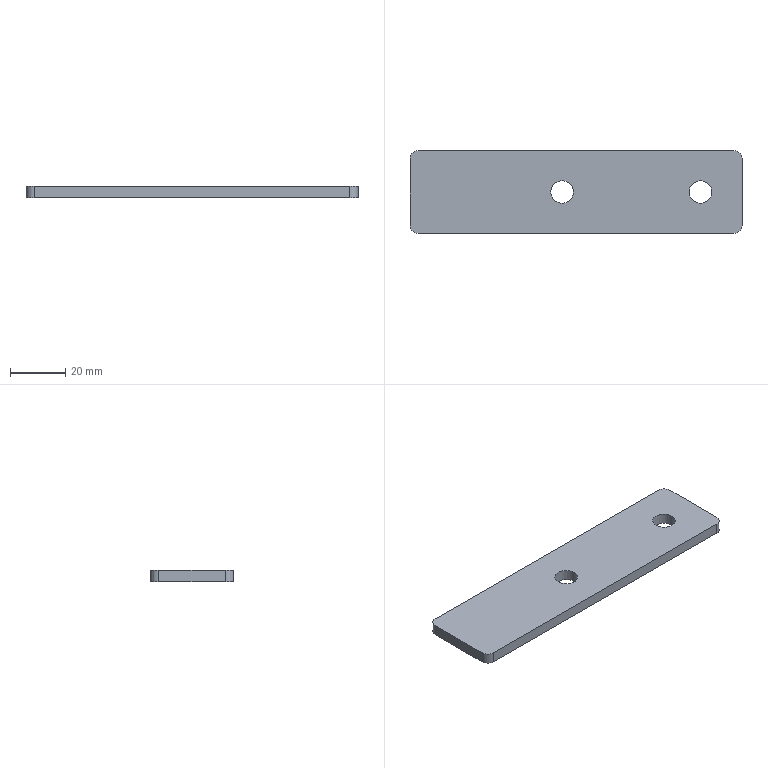Part | STEP file | Mounting bumper | 1 solid | 12 faces | box 120 x 30 x 4 mm | volume 13947 mm3 | cylinder 6 | plane 6 | commonest cylinder face diameters 6 x4 8.2 x2
STEP:
#1=CARTESIAN_POINT('',(0.,0.,0.));
#2=DIRECTION('',(0.,0.,1.));
#3=DIRECTION('',(1.,0.,0.));
#4=AXIS2_PLACEMENT_3D('',#1,#2,#3);
#5=CARTESIAN_POINT('',(109.1,15.,0.));
#6=VERTEX_POINT('',#5);
#7=CARTESIAN_POINT('',(105.,15.,0.));
#8=DIRECTION('',(0.,0.,1.));
#9=DIRECTION('',(-1.,0.,0.));
#10=AXIS2_PLACEMENT_3D('',#7,#8,#9);
#11=CIRCLE('',#10,4.1);
#12=CARTESIAN_POINT('',(105.,15.,4.));
#13=DIRECTION('',(0.,0.,-1.));
#14=DIRECTION('',(-1.,0.,0.));
#15=AXIS2_PLACEMENT_3D('',#12,#13,#14);
#16=CYLINDRICAL_SURFACE('',#15,4.1);
#17=CARTESIAN_POINT('',(12.566,4.));
#18=DIRECTION('',(-1.,0.));
#19=VECTOR('',#18,1.);
#20=LINE('',#17,#19);
#21=(GEOMETRIC_REPRESENTATION_CONTEXT(2)PARAMETRIC_REPRESENTATION_CONTEXT()REPRESENTATION_CONTEXT('',''));
#22=DEFINITIONAL_REPRESENTATION('',(#20),#21);
#23=PCURVE('',#16,#22);
#24=CARTESIAN_POINT('',(60.,15.,0.));
#25=DIRECTION('',(0.,0.,1.));
#26=DIRECTION('',(1.,0.,0.));
#27=AXIS2_PLACEMENT_3D('',#24,#25,#26);
#28=PLANE('',#27);
#29=CARTESIAN_POINT('',(45.,0.));
#30=DIRECTION('',(-1.,0.));
#31=AXIS2_PLACEMENT_2D('',#29,#30);
#32=CIRCLE('',#31,4.1);
#33=(GEOMETRIC_REPRESENTATION_CONTEXT(2)PARAMETRIC_REPRESENTATION_CONTEXT()REPRESENTATION_CONTEXT('',''));
#34=DEFINITIONAL_REPRESENTATION('',(#32),#33);
#35=PCURVE('',#28,#34);
#36=SURFACE_CURVE('',#11,(#23,#35),.PCURVE_S1.);
#37=EDGE_CURVE('',#6,#6,#36,.T.);
#38=ORIENTED_EDGE('',*,*,#37,.T.);
#39=CARTESIAN_POINT('',(109.1,15.,4.));
#40=VERTEX_POINT('',#39);
#41=CARTESIAN_POINT('',(109.1,15.,4.));
#42=CARTESIAN_POINT('',(109.1,15.,0.));
#43=B_SPLINE_CURVE_WITH_KNOTS('',1,(#41,#42),.UNSPECIFIED.,.F.,.F.,(2,2),(0.,4.),.PIECEWISE_BEZIER_KNOTS.);
#44=CARTESIAN_POINT('',(3.142,0.));
#45=DIRECTION('',(0.,1.));
#46=VECTOR('',#45,1.);
#47=LINE('',#44,#46);
#48=(GEOMETRIC_REPRESENTATION_CONTEXT(2)PARAMETRIC_REPRESENTATION_CONTEXT()REPRESENTATION_CONTEXT('',''));
#49=DEFINITIONAL_REPRESENTATION('',(#47),#48);
#50=PCURVE('',#16,#49);
#51=CARTESIAN_POINT('',(9.425,0.));
#52=DIRECTION('',(0.,1.));
#53=VECTOR('',#52,1.);
#54=LINE('',#51,#53);
#55=(GEOMETRIC_REPRESENTATION_CONTEXT(2)PARAMETRIC_REPRESENTATION_CONTEXT()REPRESENTATION_CONTEXT('',''));
#56=DEFINITIONAL_REPRESENTATION('',(#54),#55);
#57=PCURVE('',#16,#56);
#58=SEAM_CURVE('',#43,(#50,#57),.PCURVE_S1.);
#59=EDGE_CURVE('',#40,#6,#58,.T.);
#60=ORIENTED_EDGE('',*,*,#59,.F.);
#61=CARTESIAN_POINT('',(105.,15.,4.));
#62=DIRECTION('',(0.,0.,-1.));
#63=DIRECTION('',(-1.,0.,0.));
#64=AXIS2_PLACEMENT_3D('',#61,#62,#63);
#65=CIRCLE('',#64,4.1);
#66=CARTESIAN_POINT('',(0.,0.));
#67=DIRECTION('',(1.,0.));
#68=VECTOR('',#67,1.);
#69=LINE('',#66,#68);
#70=(GEOMETRIC_REPRESENTATION_CONTEXT(2)PARAMETRIC_REPRESENTATION_CONTEXT()REPRESENTATION_CONTEXT('',''));
#71=DEFINITIONAL_REPRESENTATION('',(#69),#70);
#72=PCURVE('',#16,#71);
#73=CARTESIAN_POINT('',(60.,15.,4.));
#74=DIRECTION('',(0.,0.,1.));
#75=DIRECTION('',(1.,0.,0.));
#76=AXIS2_PLACEMENT_3D('',#73,#74,#75);
#77=PLANE('',#76);
#78=CARTESIAN_POINT('',(40.9,0.));
#79=CARTESIAN_POINT('',(40.9,7.101));
#80=CARTESIAN_POINT('',(47.05,3.551));
#81=CARTESIAN_POINT('',(53.2,0.));
#82=CARTESIAN_POINT('',(47.05,-3.551));
#83=CARTESIAN_POINT('',(40.9,-7.101));
#84=CARTESIAN_POINT('',(40.9,0.));
#85=(BOUNDED_CURVE()B_SPLINE_CURVE(2,(#78,#79,#80,#81,#82,#83,#84),.UNSPECIFIED.,.T.,.F.)B_SPLINE_CURVE_WITH_KNOTS((1,2,2,2,2,1),(-2.094,0.,2.094,4.189,6.283,8.378),.UNSPECIFIED.)CURVE()GEOMETRIC_REPRESENTATION_ITEM()RATIONAL_B_SPLINE_CURVE((1.,0.5,1.,0.5,1.,0.5,1.))REPRESENTATION_ITEM(''));
#86=(GEOMETRIC_REPRESENTATION_CONTEXT(2)PARAMETRIC_REPRESENTATION_CONTEXT()REPRESENTATION_CONTEXT('',''));
#87=DEFINITIONAL_REPRESENTATION('',(#85),#86);
#88=PCURVE('',#77,#87);
#89=SURFACE_CURVE('',#65,(#72,#88),.PCURVE_S1.);
#90=EDGE_CURVE('',#40,#40,#89,.T.);
#91=ORIENTED_EDGE('',*,*,#90,.T.);
#92=ORIENTED_EDGE('',*,*,#59,.T.);
#93=EDGE_LOOP('',(#38,#60,#91,#92));
#94=FACE_BOUND('',#93,.F.);
#95=ADVANCED_FACE('',(#94),#16,.F.);
#96=CARTESIAN_POINT('',(59.1,15.,0.));
#97=VERTEX_POINT('',#96);
#98=CARTESIAN_POINT('',(55.,15.,0.));
#99=DIRECTION('',(0.,0.,1.));
#100=DIRECTION('',(-1.,0.,0.));
#101=AXIS2_PLACEMENT_3D('',#98,#99,#100);
#102=CIRCLE('',#101,4.1);
#103=CARTESIAN_POINT('',(55.,15.,4.));
#104=DIRECTION('',(0.,0.,-1.));
#105=DIRECTION('',(-1.,0.,0.));
#106=AXIS2_PLACEMENT_3D('',#103,#104,#105);
#107=CYLINDRICAL_SURFACE('',#106,4.1);
#108=CARTESIAN_POINT('',(12.566,4.));
#109=DIRECTION('',(-1.,0.));
#110=VECTOR('',#109,1.);
#111=LINE('',#108,#110);
#112=(GEOMETRIC_REPRESENTATION_CONTEXT(2)PARAMETRIC_REPRESENTATION_CONTEXT()REPRESENTATION_CONTEXT('',''));
#113=DEFINITIONAL_REPRESENTATION('',(#111),#112);
#114=PCURVE('',#107,#113);
#115=CARTESIAN_POINT('',(-5.,0.));
#116=DIRECTION('',(-1.,0.));
#117=AXIS2_PLACEMENT_2D('',#115,#116);
#118=CIRCLE('',#117,4.1);
#119=(GEOMETRIC_REPRESENTATION_CONTEXT(2)PARAMETRIC_REPRESENTATION_CONTEXT()REPRESENTATION_CONTEXT('',''));
#120=DEFINITIONAL_REPRESENTATION('',(#118),#119);
#121=PCURVE('',#28,#120);
#122=SURFACE_CURVE('',#102,(#114,#121),.PCURVE_S1.);
#123=EDGE_CURVE('',#97,#97,#122,.T.);
#124=ORIENTED_EDGE('',*,*,#123,.T.);
#125=CARTESIAN_POINT('',(59.1,15.,4.));
#126=VERTEX_POINT('',#125);
#127=CARTESIAN_POINT('',(59.1,15.,4.));
#128=CARTESIAN_POINT('',(59.1,15.,0.));
#129=B_SPLINE_CURVE_WITH_KNOTS('',1,(#127,#128),.UNSPECIFIED.,.F.,.F.,(2,2),(0.,4.),.PIECEWISE_BEZIER_KNOTS.);
#130=CARTESIAN_POINT('',(3.142,0.));
#131=DIRECTION('',(0.,1.));
#132=VECTOR('',#131,1.);
#133=LINE('',#130,#132);
#134=(GEOMETRIC_REPRESENTATION_CONTEXT(2)PARAMETRIC_REPRESENTATION_CONTEXT()REPRESENTATION_CONTEXT('',''));
#135=DEFINITIONAL_REPRESENTATION('',(#133),#134);
#136=PCURVE('',#107,#135);
#137=CARTESIAN_POINT('',(9.425,0.));
#138=DIRECTION('',(0.,1.));
#139=VECTOR('',#138,1.);
#140=LINE('',#137,#139);
#141=(GEOMETRIC_REPRESENTATION_CONTEXT(2)PARAMETRIC_REPRESENTATION_CONTEXT()REPRESENTATION_CONTEXT('',''));
#142=DEFINITIONAL_REPRESENTATION('',(#140),#141);
#143=PCURVE('',#107,#142);
#144=SEAM_CURVE('',#129,(#136,#143),.PCURVE_S1.);
#145=EDGE_CURVE('',#126,#97,#144,.T.);
#146=ORIENTED_EDGE('',*,*,#145,.F.);
#147=CARTESIAN_POINT('',(55.,15.,4.));
#148=DIRECTION('',(0.,0.,-1.));
#149=DIRECTION('',(-1.,0.,0.));
#150=AXIS2_PLACEMENT_3D('',#147,#148,#149);
#151=CIRCLE('',#150,4.1);
#152=CARTESIAN_POINT('',(0.,0.));
#153=DIRECTION('',(1.,0.));
#154=VECTOR('',#153,1.);
#155=LINE('',#152,#154);
#156=(GEOMETRIC_REPRESENTATION_CONTEXT(2)PARAMETRIC_REPRESENTATION_CONTEXT()REPRESENTATION_CONTEXT('',''));
#157=DEFINITIONAL_REPRESENTATION('',(#155),#156);
#158=PCURVE('',#107,#157);
#159=CARTESIAN_POINT('',(-9.1,0.));
#160=CARTESIAN_POINT('',(-9.1,7.101));
#161=CARTESIAN_POINT('',(-2.95,3.551));
#162=CARTESIAN_POINT('',(3.2,0.));
#163=CARTESIAN_POINT('',(-2.95,-3.551));
#164=CARTESIAN_POINT('',(-9.1,-7.101));
#165=CARTESIAN_POINT('',(-9.1,0.));
#166=(BOUNDED_CURVE()B_SPLINE_CURVE(2,(#159,#160,#161,#162,#163,#164,#165),.UNSPECIFIED.,.T.,.F.)B_SPLINE_CURVE_WITH_KNOTS((1,2,2,2,2,1),(-2.094,0.,2.094,4.189,6.283,8.378),.UNSPECIFIED.)CURVE()GEOMETRIC_REPRESENTATION_ITEM()RATIONAL_B_SPLINE_CURVE((1.,0.5,1.,0.5,1.,0.5,1.))REPRESENTATION_ITEM(''));
#167=(GEOMETRIC_REPRESENTATION_CONTEXT(2)PARAMETRIC_REPRESENTATION_CONTEXT()REPRESENTATION_CONTEXT('',''));
#168=DEFINITIONAL_REPRESENTATION('',(#166),#167);
#169=PCURVE('',#77,#168);
#170=SURFACE_CURVE('',#151,(#158,#169),.PCURVE_S1.);
#171=EDGE_CURVE('',#126,#126,#170,.T.);
#172=ORIENTED_EDGE('',*,*,#171,.T.);
#173=ORIENTED_EDGE('',*,*,#145,.T.);
#174=EDGE_LOOP('',(#124,#146,#172,#173));
#175=FACE_BOUND('',#174,.F.);
#176=ADVANCED_FACE('',(#175),#107,.F.);
#177=CARTESIAN_POINT('',(120.,3.,4.));
#178=VERTEX_POINT('',#177);
#179=CARTESIAN_POINT('',(117.,0.,4.));
#180=VERTEX_POINT('',#179);
#181=CARTESIAN_POINT('',(117.,3.,4.));
#182=DIRECTION('',(0.,0.,-1.));
#183=DIRECTION('',(0.7071,-0.7071,0.));
#184=AXIS2_PLACEMENT_3D('',#181,#182,#183);
#185=CIRCLE('',#184,3.);
#186=CARTESIAN_POINT('',(117.,3.,0.));
#187=DIRECTION('',(0.,0.,1.));
#188=DIRECTION('',(0.7071,-0.7071,0.));
#189=AXIS2_PLACEMENT_3D('',#186,#187,#188);
#190=CYLINDRICAL_SURFACE('',#189,3.);
#191=CARTESIAN_POINT('',(6.283,4.));
#192=DIRECTION('',(-1.,0.));
#193=VECTOR('',#192,1.);
#194=LINE('',#191,#193);
#195=(GEOMETRIC_REPRESENTATION_CONTEXT(2)PARAMETRIC_REPRESENTATION_CONTEXT()REPRESENTATION_CONTEXT('',''));
#196=DEFINITIONAL_REPRESENTATION('',(#194),#195);
#197=PCURVE('',#190,#196);
#198=CARTESIAN_POINT('',(59.121,-14.121));
#199=CARTESIAN_POINT('',(55.447,-17.796));
#200=CARTESIAN_POINT('',(54.102,-12.776));
#201=CARTESIAN_POINT('',(52.757,-7.757));
#202=CARTESIAN_POINT('',(57.776,-9.102));
#203=CARTESIAN_POINT('',(62.796,-10.447));
#204=CARTESIAN_POINT('',(59.121,-14.121));
#205=(BOUNDED_CURVE()B_SPLINE_CURVE(2,(#198,#199,#200,#201,#202,#203,#204),.UNSPECIFIED.,.T.,.F.)B_SPLINE_CURVE_WITH_KNOTS((1,2,2,2,2,1),(-2.094,0.,2.094,4.189,6.283,8.378),.UNSPECIFIED.)CURVE()GEOMETRIC_REPRESENTATION_ITEM()RATIONAL_B_SPLINE_CURVE((1.,0.5,1.,0.5,1.,0.5,1.))REPRESENTATION_ITEM(''));
#206=(GEOMETRIC_REPRESENTATION_CONTEXT(2)PARAMETRIC_REPRESENTATION_CONTEXT()REPRESENTATION_CONTEXT('',''));
#207=DEFINITIONAL_REPRESENTATION('',(#205),#206);
#208=PCURVE('',#77,#207);
#209=SURFACE_CURVE('',#185,(#197,#208),.PCURVE_S1.);
#210=EDGE_CURVE('',#178,#180,#209,.T.);
#211=ORIENTED_EDGE('',*,*,#210,.T.);
#212=CARTESIAN_POINT('',(117.,0.,0.));
#213=VERTEX_POINT('',#212);
#214=CARTESIAN_POINT('',(117.,0.,0.));
#215=DIRECTION('',(0.,0.,-1.));
#216=VECTOR('',#215,1.);
#217=LINE('',#214,#216);
#218=CARTESIAN_POINT('',(-0.7854,0.));
#219=DIRECTION('',(0.,-1.));
#220=VECTOR('',#219,1.);
#221=LINE('',#218,#220);
#222=(GEOMETRIC_REPRESENTATION_CONTEXT(2)PARAMETRIC_REPRESENTATION_CONTEXT()REPRESENTATION_CONTEXT('',''));
#223=DEFINITIONAL_REPRESENTATION('',(#221),#222);
#224=PCURVE('',#190,#223);
#225=CARTESIAN_POINT('',(120.,0.,0.));
#226=DIRECTION('',(0.,-1.,0.));
#227=DIRECTION('',(0.,0.,-1.));
#228=AXIS2_PLACEMENT_3D('',#225,#226,#227);
#229=PLANE('',#228);
#230=CARTESIAN_POINT('',(0.,-3.));
#231=DIRECTION('',(1.,0.));
#232=VECTOR('',#231,1.);
#233=LINE('',#230,#232);
#234=(GEOMETRIC_REPRESENTATION_CONTEXT(2)PARAMETRIC_REPRESENTATION_CONTEXT()REPRESENTATION_CONTEXT('',''));
#235=DEFINITIONAL_REPRESENTATION('',(#233),#234);
#236=PCURVE('',#229,#235);
#237=SURFACE_CURVE('',#217,(#224,#236),.PCURVE_S1.);
#238=EDGE_CURVE('',#180,#213,#237,.T.);
#239=ORIENTED_EDGE('',*,*,#238,.T.);
#240=CARTESIAN_POINT('',(120.,3.,0.));
#241=VERTEX_POINT('',#240);
#242=CARTESIAN_POINT('',(117.,3.,0.));
#243=DIRECTION('',(0.,0.,1.));
#244=DIRECTION('',(0.7071,-0.7071,0.));
#245=AXIS2_PLACEMENT_3D('',#242,#243,#244);
#246=CIRCLE('',#245,3.);
#247=CARTESIAN_POINT('',(-6.283,0.));
#248=DIRECTION('',(1.,0.));
#249=VECTOR('',#248,1.);
#250=LINE('',#247,#249);
#251=(GEOMETRIC_REPRESENTATION_CONTEXT(2)PARAMETRIC_REPRESENTATION_CONTEXT()REPRESENTATION_CONTEXT('',''));
#252=DEFINITIONAL_REPRESENTATION('',(#250),#251);
#253=PCURVE('',#190,#252);
#254=CARTESIAN_POINT('',(57.,-12.));
#255=DIRECTION('',(0.7071,-0.7071));
#256=AXIS2_PLACEMENT_2D('',#254,#255);
#257=CIRCLE('',#256,3.);
#258=(GEOMETRIC_REPRESENTATION_CONTEXT(2)PARAMETRIC_REPRESENTATION_CONTEXT()REPRESENTATION_CONTEXT('',''));
#259=DEFINITIONAL_REPRESENTATION('',(#257),#258);
#260=PCURVE('',#28,#259);
#261=SURFACE_CURVE('',#246,(#253,#260),.PCURVE_S1.);
#262=EDGE_CURVE('',#213,#241,#261,.T.);
#263=ORIENTED_EDGE('',*,*,#262,.T.);
#264=CARTESIAN_POINT('',(120.,3.,0.));
#265=DIRECTION('',(0.,0.,1.));
#266=VECTOR('',#265,1.);
#267=LINE('',#264,#266);
#268=CARTESIAN_POINT('',(0.7854,0.));
#269=DIRECTION('',(0.,1.));
#270=VECTOR('',#269,1.);
#271=LINE('',#268,#270);
#272=(GEOMETRIC_REPRESENTATION_CONTEXT(2)PARAMETRIC_REPRESENTATION_CONTEXT()REPRESENTATION_CONTEXT('',''));
#273=DEFINITIONAL_REPRESENTATION('',(#271),#272);
#274=PCURVE('',#190,#273);
#275=CARTESIAN_POINT('',(120.,30.,0.));
#276=DIRECTION('',(1.,0.,0.));
#277=DIRECTION('',(0.,0.,-1.));
#278=AXIS2_PLACEMENT_3D('',#275,#276,#277);
#279=PLANE('',#278);
#280=CARTESIAN_POINT('',(0.,-27.));
#281=DIRECTION('',(-1.,0.));
#282=VECTOR('',#281,1.);
#283=LINE('',#280,#282);
#284=(GEOMETRIC_REPRESENTATION_CONTEXT(2)PARAMETRIC_REPRESENTATION_CONTEXT()REPRESENTATION_CONTEXT('',''));
#285=DEFINITIONAL_REPRESENTATION('',(#283),#284);
#286=PCURVE('',#279,#285);
#287=SURFACE_CURVE('',#267,(#274,#286),.PCURVE_S1.);
#288=EDGE_CURVE('',#241,#178,#287,.T.);
#289=ORIENTED_EDGE('',*,*,#288,.T.);
#290=EDGE_LOOP('',(#211,#239,#263,#289));
#291=FACE_BOUND('',#290,.T.);
#292=ADVANCED_FACE('',(#291),#190,.T.);
#293=ORIENTED_EDGE('',*,*,#288,.F.);
#294=CARTESIAN_POINT('',(120.,27.,0.));
#295=VERTEX_POINT('',#294);
#296=CARTESIAN_POINT('',(120.,30.,0.));
#297=DIRECTION('',(0.,-1.,0.));
#298=VECTOR('',#297,1.);
#299=LINE('',#296,#298);
#300=CARTESIAN_POINT('',(0.,0.));
#301=DIRECTION('',(0.,-1.));
#302=VECTOR('',#301,1.);
#303=LINE('',#300,#302);
#304=(GEOMETRIC_REPRESENTATION_CONTEXT(2)PARAMETRIC_REPRESENTATION_CONTEXT()REPRESENTATION_CONTEXT('',''));
#305=DEFINITIONAL_REPRESENTATION('',(#303),#304);
#306=PCURVE('',#279,#305);
#307=CARTESIAN_POINT('',(60.,15.));
#308=DIRECTION('',(0.,-1.));
#309=VECTOR('',#308,1.);
#310=LINE('',#307,#309);
#311=(GEOMETRIC_REPRESENTATION_CONTEXT(2)PARAMETRIC_REPRESENTATION_CONTEXT()REPRESENTATION_CONTEXT('',''));
#312=DEFINITIONAL_REPRESENTATION('',(#310),#311);
#313=PCURVE('',#28,#312);
#314=SURFACE_CURVE('',#299,(#306,#313),.PCURVE_S1.);
#315=EDGE_CURVE('',#295,#241,#314,.T.);
#316=ORIENTED_EDGE('',*,*,#315,.F.);
#317=CARTESIAN_POINT('',(120.,27.,4.));
#318=VERTEX_POINT('',#317);
#319=CARTESIAN_POINT('',(120.,27.,0.));
#320=DIRECTION('',(0.,0.,-1.));
#321=VECTOR('',#320,1.);
#322=LINE('',#319,#321);
#323=CARTESIAN_POINT('',(0.,-3.));
#324=DIRECTION('',(1.,0.));
#325=VECTOR('',#324,1.);
#326=LINE('',#323,#325);
#327=(GEOMETRIC_REPRESENTATION_CONTEXT(2)PARAMETRIC_REPRESENTATION_CONTEXT()REPRESENTATION_CONTEXT('',''));
#328=DEFINITIONAL_REPRESENTATION('',(#326),#327);
#329=PCURVE('',#279,#328);
#330=CARTESIAN_POINT('',(117.,27.,0.));
#331=DIRECTION('',(0.,0.,1.));
#332=DIRECTION('',(0.7071,0.7071,0.));
#333=AXIS2_PLACEMENT_3D('',#330,#331,#332);
#334=CYLINDRICAL_SURFACE('',#333,3.);
#335=CARTESIAN_POINT('',(-0.7854,0.));
#336=DIRECTION('',(0.,-1.));
#337=VECTOR('',#336,1.);
#338=LINE('',#335,#337);
#339=(GEOMETRIC_REPRESENTATION_CONTEXT(2)PARAMETRIC_REPRESENTATION_CONTEXT()REPRESENTATION_CONTEXT('',''));
#340=DEFINITIONAL_REPRESENTATION('',(#338),#339);
#341=PCURVE('',#334,#340);
#342=SURFACE_CURVE('',#322,(#329,#341),.PCURVE_S1.);
#343=EDGE_CURVE('',#318,#295,#342,.T.);
#344=ORIENTED_EDGE('',*,*,#343,.F.);
#345=CARTESIAN_POINT('',(120.,30.,4.));
#346=DIRECTION('',(0.,-1.,0.));
#347=VECTOR('',#346,1.);
#348=LINE('',#345,#347);
#349=CARTESIAN_POINT('',(-4.,0.));
#350=DIRECTION('',(0.,-1.));
#351=VECTOR('',#350,1.);
#352=LINE('',#349,#351);
#353=(GEOMETRIC_REPRESENTATION_CONTEXT(2)PARAMETRIC_REPRESENTATION_CONTEXT()REPRESENTATION_CONTEXT('',''));
#354=DEFINITIONAL_REPRESENTATION('',(#352),#353);
#355=PCURVE('',#279,#354);
#356=CARTESIAN_POINT('',(60.,15.));
#357=DIRECTION('',(0.,-1.));
#358=VECTOR('',#357,1.);
#359=LINE('',#356,#358);
#360=(GEOMETRIC_REPRESENTATION_CONTEXT(2)PARAMETRIC_REPRESENTATION_CONTEXT()REPRESENTATION_CONTEXT('',''));
#361=DEFINITIONAL_REPRESENTATION('',(#359),#360);
#362=PCURVE('',#77,#361);
#363=SURFACE_CURVE('',#348,(#355,#362),.PCURVE_S1.);
#364=EDGE_CURVE('',#318,#178,#363,.T.);
#365=ORIENTED_EDGE('',*,*,#364,.T.);
#366=EDGE_LOOP('',(#293,#316,#344,#365));
#367=FACE_BOUND('',#366,.T.);
#368=ADVANCED_FACE('',(#367),#279,.T.);
#369=ORIENTED_EDGE('',*,*,#262,.F.);
#370=CARTESIAN_POINT('',(3.,0.,0.));
#371=VERTEX_POINT('',#370);
#372=CARTESIAN_POINT('',(120.,0.,0.));
#373=DIRECTION('',(-1.,0.,0.));
#374=VECTOR('',#373,1.);
#375=LINE('',#372,#374);
#376=CARTESIAN_POINT('',(60.,-15.));
#377=DIRECTION('',(-1.,0.));
#378=VECTOR('',#377,1.);
#379=LINE('',#376,#378);
#380=(GEOMETRIC_REPRESENTATION_CONTEXT(2)PARAMETRIC_REPRESENTATION_CONTEXT()REPRESENTATION_CONTEXT('',''));
#381=DEFINITIONAL_REPRESENTATION('',(#379),#380);
#382=PCURVE('',#28,#381);
#383=CARTESIAN_POINT('',(0.,0.));
#384=DIRECTION('',(0.,-1.));
#385=VECTOR('',#384,1.);
#386=LINE('',#383,#385);
#387=(GEOMETRIC_REPRESENTATION_CONTEXT(2)PARAMETRIC_REPRESENTATION_CONTEXT()REPRESENTATION_CONTEXT('',''));
#388=DEFINITIONAL_REPRESENTATION('',(#386),#387);
#389=PCURVE('',#229,#388);
#390=SURFACE_CURVE('',#375,(#382,#389),.PCURVE_S1.);
#391=EDGE_CURVE('',#213,#371,#390,.T.);
#392=ORIENTED_EDGE('',*,*,#391,.T.);
#393=CARTESIAN_POINT('',(0.,3.,0.));
#394=VERTEX_POINT('',#393);
#395=CARTESIAN_POINT('',(3.,3.,0.));
#396=DIRECTION('',(0.,0.,1.));
#397=DIRECTION('',(-0.7071,-0.7071,0.));
#398=AXIS2_PLACEMENT_3D('',#395,#396,#397);
#399=CIRCLE('',#398,3.);
#400=CARTESIAN_POINT('',(-57.,-12.));
#401=DIRECTION('',(-0.7071,-0.7071));
#402=AXIS2_PLACEMENT_2D('',#400,#401);
#403=CIRCLE('',#402,3.);
#404=(GEOMETRIC_REPRESENTATION_CONTEXT(2)PARAMETRIC_REPRESENTATION_CONTEXT()REPRESENTATION_CONTEXT('',''));
#405=DEFINITIONAL_REPRESENTATION('',(#403),#404);
#406=PCURVE('',#28,#405);
#407=CARTESIAN_POINT('',(3.,3.,0.));
#408=DIRECTION('',(0.,0.,1.));
#409=DIRECTION('',(-0.7071,-0.7071,0.));
#410=AXIS2_PLACEMENT_3D('',#407,#408,#409);
#411=CYLINDRICAL_SURFACE('',#410,3.);
#412=CARTESIAN_POINT('',(-6.283,0.));
#413=DIRECTION('',(1.,0.));
#414=VECTOR('',#413,1.);
#415=LINE('',#412,#414);
#416=(GEOMETRIC_REPRESENTATION_CONTEXT(2)PARAMETRIC_REPRESENTATION_CONTEXT()REPRESENTATION_CONTEXT('',''));
#417=DEFINITIONAL_REPRESENTATION('',(#415),#416);
#418=PCURVE('',#411,#417);
#419=SURFACE_CURVE('',#399,(#406,#418),.PCURVE_S1.);
#420=EDGE_CURVE('',#394,#371,#419,.T.);
#421=ORIENTED_EDGE('',*,*,#420,.F.);
#422=CARTESIAN_POINT('',(0.,27.,0.));
#423=VERTEX_POINT('',#422);
#424=CARTESIAN_POINT('',(0.,0.,0.));
#425=DIRECTION('',(0.,1.,0.));
#426=VECTOR('',#425,1.);
#427=LINE('',#424,#426);
#428=CARTESIAN_POINT('',(-60.,-15.));
#429=DIRECTION('',(0.,1.));
#430=VECTOR('',#429,1.);
#431=LINE('',#428,#430);
#432=(GEOMETRIC_REPRESENTATION_CONTEXT(2)PARAMETRIC_REPRESENTATION_CONTEXT()REPRESENTATION_CONTEXT('',''));
#433=DEFINITIONAL_REPRESENTATION('',(#431),#432);
#434=PCURVE('',#28,#433);
#435=CARTESIAN_POINT('',(0.,0.,0.));
#436=DIRECTION('',(-1.,0.,0.));
#437=DIRECTION('',(0.,0.,1.));
#438=AXIS2_PLACEMENT_3D('',#435,#436,#437);
#439=PLANE('',#438);
#440=CARTESIAN_POINT('',(0.,0.));
#441=DIRECTION('',(0.,1.));
#442=VECTOR('',#441,1.);
#443=LINE('',#440,#442);
#444=(GEOMETRIC_REPRESENTATION_CONTEXT(2)PARAMETRIC_REPRESENTATION_CONTEXT()REPRESENTATION_CONTEXT('',''));
#445=DEFINITIONAL_REPRESENTATION('',(#443),#444);
#446=PCURVE('',#439,#445);
#447=SURFACE_CURVE('',#427,(#434,#446),.PCURVE_S1.);
#448=EDGE_CURVE('',#394,#423,#447,.T.);
#449=ORIENTED_EDGE('',*,*,#448,.T.);
#450=CARTESIAN_POINT('',(3.,30.,0.));
#451=VERTEX_POINT('',#450);
#452=CARTESIAN_POINT('',(3.,27.,0.));
#453=DIRECTION('',(0.,0.,1.));
#454=DIRECTION('',(-0.7071,0.7071,0.));
#455=AXIS2_PLACEMENT_3D('',#452,#453,#454);
#456=CIRCLE('',#455,3.);
#457=CARTESIAN_POINT('',(-57.,12.));
#458=DIRECTION('',(-0.7071,0.7071));
#459=AXIS2_PLACEMENT_2D('',#457,#458);
#460=CIRCLE('',#459,3.);
#461=(GEOMETRIC_REPRESENTATION_CONTEXT(2)PARAMETRIC_REPRESENTATION_CONTEXT()REPRESENTATION_CONTEXT('',''));
#462=DEFINITIONAL_REPRESENTATION('',(#460),#461);
#463=PCURVE('',#28,#462);
#464=CARTESIAN_POINT('',(3.,27.,0.));
#465=DIRECTION('',(0.,0.,1.));
#466=DIRECTION('',(-0.7071,0.7071,0.));
#467=AXIS2_PLACEMENT_3D('',#464,#465,#466);
#468=CYLINDRICAL_SURFACE('',#467,3.);
#469=CARTESIAN_POINT('',(0.,0.));
#470=DIRECTION('',(1.,0.));
#471=VECTOR('',#470,1.);
#472=LINE('',#469,#471);
#473=(GEOMETRIC_REPRESENTATION_CONTEXT(2)PARAMETRIC_REPRESENTATION_CONTEXT()REPRESENTATION_CONTEXT('',''));
#474=DEFINITIONAL_REPRESENTATION('',(#472),#473);
#475=PCURVE('',#468,#474);
#476=SURFACE_CURVE('',#456,(#463,#475),.PCURVE_S1.);
#477=EDGE_CURVE('',#451,#423,#476,.T.);
#478=ORIENTED_EDGE('',*,*,#477,.F.);
#479=CARTESIAN_POINT('',(117.,30.,0.));
#480=VERTEX_POINT('',#479);
#481=CARTESIAN_POINT('',(0.,30.,0.));
#482=DIRECTION('',(1.,0.,0.));
#483=VECTOR('',#482,1.);
#484=LINE('',#481,#483);
#485=CARTESIAN_POINT('',(-60.,15.));
#486=DIRECTION('',(1.,0.));
#487=VECTOR('',#486,1.);
#488=LINE('',#485,#487);
#489=(GEOMETRIC_REPRESENTATION_CONTEXT(2)PARAMETRIC_REPRESENTATION_CONTEXT()REPRESENTATION_CONTEXT('',''));
#490=DEFINITIONAL_REPRESENTATION('',(#488),#489);
#491=PCURVE('',#28,#490);
#492=CARTESIAN_POINT('',(30.,30.,0.));
#493=DIRECTION('',(0.,1.,0.));
#494=DIRECTION('',(0.,0.,1.));
#495=AXIS2_PLACEMENT_3D('',#492,#493,#494);
#496=PLANE('',#495);
#497=CARTESIAN_POINT('',(0.,-30.));
#498=DIRECTION('',(0.,1.));
#499=VECTOR('',#498,1.);
#500=LINE('',#497,#499);
#501=(GEOMETRIC_REPRESENTATION_CONTEXT(2)PARAMETRIC_REPRESENTATION_CONTEXT()REPRESENTATION_CONTEXT('',''));
#502=DEFINITIONAL_REPRESENTATION('',(#500),#501);
#503=PCURVE('',#496,#502);
#504=SURFACE_CURVE('',#484,(#491,#503),.PCURVE_S1.);
#505=EDGE_CURVE('',#451,#480,#504,.T.);
#506=ORIENTED_EDGE('',*,*,#505,.T.);
#507=CARTESIAN_POINT('',(117.,27.,0.));
#508=DIRECTION('',(0.,0.,1.));
#509=DIRECTION('',(0.7071,0.7071,0.));
#510=AXIS2_PLACEMENT_3D('',#507,#508,#509);
#511=CIRCLE('',#510,3.);
#512=CARTESIAN_POINT('',(57.,12.));
#513=DIRECTION('',(0.7071,0.7071));
#514=AXIS2_PLACEMENT_2D('',#512,#513);
#515=CIRCLE('',#514,3.);
#516=(GEOMETRIC_REPRESENTATION_CONTEXT(2)PARAMETRIC_REPRESENTATION_CONTEXT()REPRESENTATION_CONTEXT('',''));
#517=DEFINITIONAL_REPRESENTATION('',(#515),#516);
#518=PCURVE('',#28,#517);
#519=CARTESIAN_POINT('',(-6.283,0.));
#520=DIRECTION('',(1.,0.));
#521=VECTOR('',#520,1.);
#522=LINE('',#519,#521);
#523=(GEOMETRIC_REPRESENTATION_CONTEXT(2)PARAMETRIC_REPRESENTATION_CONTEXT()REPRESENTATION_CONTEXT('',''));
#524=DEFINITIONAL_REPRESENTATION('',(#522),#523);
#525=PCURVE('',#334,#524);
#526=SURFACE_CURVE('',#511,(#518,#525),.PCURVE_S1.);
#527=EDGE_CURVE('',#295,#480,#526,.T.);
#528=ORIENTED_EDGE('',*,*,#527,.F.);
#529=ORIENTED_EDGE('',*,*,#315,.T.);
#530=EDGE_LOOP('',(#369,#392,#421,#449,#478,#506,#528,#529));
#531=FACE_BOUND('',#530,.T.);
#532=ORIENTED_EDGE('',*,*,#37,.T.);
#533=EDGE_LOOP('',(#532));
#534=FACE_BOUND('',#533,.T.);
#535=ORIENTED_EDGE('',*,*,#123,.T.);
#536=EDGE_LOOP('',(#535));
#537=FACE_BOUND('',#536,.T.);
#538=ADVANCED_FACE('',(#531,#534,#537),#28,.F.);
#539=CARTESIAN_POINT('',(117.,30.,4.));
#540=VERTEX_POINT('',#539);
#541=CARTESIAN_POINT('',(117.,27.,4.));
#542=DIRECTION('',(0.,0.,-1.));
#543=DIRECTION('',(0.7071,0.7071,0.));
#544=AXIS2_PLACEMENT_3D('',#541,#542,#543);
#545=CIRCLE('',#544,3.);
#546=CARTESIAN_POINT('',(6.283,4.));
#547=DIRECTION('',(-1.,0.));
#548=VECTOR('',#547,1.);
#549=LINE('',#546,#548);
#550=(GEOMETRIC_REPRESENTATION_CONTEXT(2)PARAMETRIC_REPRESENTATION_CONTEXT()REPRESENTATION_CONTEXT('',''));
#551=DEFINITIONAL_REPRESENTATION('',(#549),#550);
#552=PCURVE('',#334,#551);
#553=CARTESIAN_POINT('',(59.121,14.121));
#554=CARTESIAN_POINT('',(62.796,10.447));
#555=CARTESIAN_POINT('',(57.776,9.102));
#556=CARTESIAN_POINT('',(52.757,7.757));
#557=CARTESIAN_POINT('',(54.102,12.776));
#558=CARTESIAN_POINT('',(55.447,17.796));
#559=CARTESIAN_POINT('',(59.121,14.121));
#560=(BOUNDED_CURVE()B_SPLINE_CURVE(2,(#553,#554,#555,#556,#557,#558,#559),.UNSPECIFIED.,.T.,.F.)B_SPLINE_CURVE_WITH_KNOTS((1,2,2,2,2,1),(-2.094,0.,2.094,4.189,6.283,8.378),.UNSPECIFIED.)CURVE()GEOMETRIC_REPRESENTATION_ITEM()RATIONAL_B_SPLINE_CURVE((1.,0.5,1.,0.5,1.,0.5,1.))REPRESENTATION_ITEM(''));
#561=(GEOMETRIC_REPRESENTATION_CONTEXT(2)PARAMETRIC_REPRESENTATION_CONTEXT()REPRESENTATION_CONTEXT('',''));
#562=DEFINITIONAL_REPRESENTATION('',(#560),#561);
#563=PCURVE('',#77,#562);
#564=SURFACE_CURVE('',#545,(#552,#563),.PCURVE_S1.);
#565=EDGE_CURVE('',#540,#318,#564,.T.);
#566=ORIENTED_EDGE('',*,*,#565,.T.);
#567=ORIENTED_EDGE('',*,*,#343,.T.);
#568=ORIENTED_EDGE('',*,*,#527,.T.);
#569=CARTESIAN_POINT('',(117.,30.,0.));
#570=DIRECTION('',(0.,0.,1.));
#571=VECTOR('',#570,1.);
#572=LINE('',#569,#571);
#573=CARTESIAN_POINT('',(0.7854,0.));
#574=DIRECTION('',(0.,1.));
#575=VECTOR('',#574,1.);
#576=LINE('',#573,#575);
#577=(GEOMETRIC_REPRESENTATION_CONTEXT(2)PARAMETRIC_REPRESENTATION_CONTEXT()REPRESENTATION_CONTEXT('',''));
#578=DEFINITIONAL_REPRESENTATION('',(#576),#577);
#579=PCURVE('',#334,#578);
#580=CARTESIAN_POINT('',(0.,87.));
#581=DIRECTION('',(1.,0.));
#582=VECTOR('',#581,1.);
#583=LINE('',#580,#582);
#584=(GEOMETRIC_REPRESENTATION_CONTEXT(2)PARAMETRIC_REPRESENTATION_CONTEXT()REPRESENTATION_CONTEXT('',''));
#585=DEFINITIONAL_REPRESENTATION('',(#583),#584);
#586=PCURVE('',#496,#585);
#587=SURFACE_CURVE('',#572,(#579,#586),.PCURVE_S1.);
#588=EDGE_CURVE('',#480,#540,#587,.T.);
#589=ORIENTED_EDGE('',*,*,#588,.T.);
#590=EDGE_LOOP('',(#566,#567,#568,#589));
#591=FACE_BOUND('',#590,.T.);
#592=ADVANCED_FACE('',(#591),#334,.T.);
#593=ORIENTED_EDGE('',*,*,#588,.F.);
#594=ORIENTED_EDGE('',*,*,#505,.F.);
#595=CARTESIAN_POINT('',(3.,30.,4.));
#596=VERTEX_POINT('',#595);
#597=CARTESIAN_POINT('',(3.,30.,0.));
#598=DIRECTION('',(0.,0.,-1.));
#599=VECTOR('',#598,1.);
#600=LINE('',#597,#599);
#601=CARTESIAN_POINT('',(0.,-27.));
#602=DIRECTION('',(-1.,0.));
#603=VECTOR('',#602,1.);
#604=LINE('',#601,#603);
#605=(GEOMETRIC_REPRESENTATION_CONTEXT(2)PARAMETRIC_REPRESENTATION_CONTEXT()REPRESENTATION_CONTEXT('',''));
#606=DEFINITIONAL_REPRESENTATION('',(#604),#605);
#607=PCURVE('',#496,#606);
#608=CARTESIAN_POINT('',(5.498,0.));
#609=DIRECTION('',(0.,-1.));
#610=VECTOR('',#609,1.);
#611=LINE('',#608,#610);
#612=(GEOMETRIC_REPRESENTATION_CONTEXT(2)PARAMETRIC_REPRESENTATION_CONTEXT()REPRESENTATION_CONTEXT('',''));
#613=DEFINITIONAL_REPRESENTATION('',(#611),#612);
#614=PCURVE('',#468,#613);
#615=SURFACE_CURVE('',#600,(#607,#614),.PCURVE_S1.);
#616=EDGE_CURVE('',#596,#451,#615,.T.);
#617=ORIENTED_EDGE('',*,*,#616,.F.);
#618=CARTESIAN_POINT('',(30.,30.,4.));
#619=DIRECTION('',(1.,0.,0.));
#620=VECTOR('',#619,1.);
#621=LINE('',#618,#620);
#622=CARTESIAN_POINT('',(4.,0.));
#623=DIRECTION('',(0.,1.));
#624=VECTOR('',#623,1.);
#625=LINE('',#622,#624);
#626=(GEOMETRIC_REPRESENTATION_CONTEXT(2)PARAMETRIC_REPRESENTATION_CONTEXT()REPRESENTATION_CONTEXT('',''));
#627=DEFINITIONAL_REPRESENTATION('',(#625),#626);
#628=PCURVE('',#496,#627);
#629=CARTESIAN_POINT('',(-30.,15.));
#630=DIRECTION('',(1.,0.));
#631=VECTOR('',#630,1.);
#632=LINE('',#629,#631);
#633=(GEOMETRIC_REPRESENTATION_CONTEXT(2)PARAMETRIC_REPRESENTATION_CONTEXT()REPRESENTATION_CONTEXT('',''));
#634=DEFINITIONAL_REPRESENTATION('',(#632),#633);
#635=PCURVE('',#77,#634);
#636=SURFACE_CURVE('',#621,(#628,#635),.PCURVE_S1.);
#637=EDGE_CURVE('',#596,#540,#636,.T.);
#638=ORIENTED_EDGE('',*,*,#637,.T.);
#639=EDGE_LOOP('',(#593,#594,#617,#638));
#640=FACE_BOUND('',#639,.T.);
#641=ADVANCED_FACE('',(#640),#496,.T.);
#642=CARTESIAN_POINT('',(0.,27.,4.));
#643=VERTEX_POINT('',#642);
#644=CARTESIAN_POINT('',(3.,27.,4.));
#645=DIRECTION('',(0.,0.,-1.));
#646=DIRECTION('',(-0.7071,0.7071,0.));
#647=AXIS2_PLACEMENT_3D('',#644,#645,#646);
#648=CIRCLE('',#647,3.);
#649=CARTESIAN_POINT('',(12.566,4.));
#650=DIRECTION('',(-1.,0.));
#651=VECTOR('',#650,1.);
#652=LINE('',#649,#651);
#653=(GEOMETRIC_REPRESENTATION_CONTEXT(2)PARAMETRIC_REPRESENTATION_CONTEXT()REPRESENTATION_CONTEXT('',''));
#654=DEFINITIONAL_REPRESENTATION('',(#652),#653);
#655=PCURVE('',#468,#654);
#656=CARTESIAN_POINT('',(-59.121,14.121));
#657=CARTESIAN_POINT('',(-55.447,17.796));
#658=CARTESIAN_POINT('',(-54.102,12.776));
#659=CARTESIAN_POINT('',(-52.757,7.757));
#660=CARTESIAN_POINT('',(-57.776,9.102));
#661=CARTESIAN_POINT('',(-62.796,10.447));
#662=CARTESIAN_POINT('',(-59.121,14.121));
#663=(BOUNDED_CURVE()B_SPLINE_CURVE(2,(#656,#657,#658,#659,#660,#661,#662),.UNSPECIFIED.,.T.,.F.)B_SPLINE_CURVE_WITH_KNOTS((1,2,2,2,2,1),(-2.094,0.,2.094,4.189,6.283,8.378),.UNSPECIFIED.)CURVE()GEOMETRIC_REPRESENTATION_ITEM()RATIONAL_B_SPLINE_CURVE((1.,0.5,1.,0.5,1.,0.5,1.))REPRESENTATION_ITEM(''));
#664=(GEOMETRIC_REPRESENTATION_CONTEXT(2)PARAMETRIC_REPRESENTATION_CONTEXT()REPRESENTATION_CONTEXT('',''));
#665=DEFINITIONAL_REPRESENTATION('',(#663),#664);
#666=PCURVE('',#77,#665);
#667=SURFACE_CURVE('',#648,(#655,#666),.PCURVE_S1.);
#668=EDGE_CURVE('',#643,#596,#667,.T.);
#669=ORIENTED_EDGE('',*,*,#668,.T.);
#670=ORIENTED_EDGE('',*,*,#616,.T.);
#671=ORIENTED_EDGE('',*,*,#477,.T.);
#672=CARTESIAN_POINT('',(0.,27.,0.));
#673=DIRECTION('',(0.,0.,1.));
#674=VECTOR('',#673,1.);
#675=LINE('',#672,#674);
#676=CARTESIAN_POINT('',(7.069,0.));
#677=DIRECTION('',(0.,1.));
#678=VECTOR('',#677,1.);
#679=LINE('',#676,#678);
#680=(GEOMETRIC_REPRESENTATION_CONTEXT(2)PARAMETRIC_REPRESENTATION_CONTEXT()REPRESENTATION_CONTEXT('',''));
#681=DEFINITIONAL_REPRESENTATION('',(#679),#680);
#682=PCURVE('',#468,#681);
#683=CARTESIAN_POINT('',(0.,27.));
#684=DIRECTION('',(1.,0.));
#685=VECTOR('',#684,1.);
#686=LINE('',#683,#685);
#687=(GEOMETRIC_REPRESENTATION_CONTEXT(2)PARAMETRIC_REPRESENTATION_CONTEXT()REPRESENTATION_CONTEXT('',''));
#688=DEFINITIONAL_REPRESENTATION('',(#686),#687);
#689=PCURVE('',#439,#688);
#690=SURFACE_CURVE('',#675,(#682,#689),.PCURVE_S1.);
#691=EDGE_CURVE('',#423,#643,#690,.T.);
#692=ORIENTED_EDGE('',*,*,#691,.T.);
#693=EDGE_LOOP('',(#669,#670,#671,#692));
#694=FACE_BOUND('',#693,.T.);
#695=ADVANCED_FACE('',(#694),#468,.T.);
#696=ORIENTED_EDGE('',*,*,#691,.F.);
#697=ORIENTED_EDGE('',*,*,#448,.F.);
#698=CARTESIAN_POINT('',(0.,3.,4.));
#699=VERTEX_POINT('',#698);
#700=CARTESIAN_POINT('',(0.,3.,0.));
#701=DIRECTION('',(0.,0.,-1.));
#702=VECTOR('',#701,1.);
#703=LINE('',#700,#702);
#704=CARTESIAN_POINT('',(0.,3.));
#705=DIRECTION('',(-1.,0.));
#706=VECTOR('',#705,1.);
#707=LINE('',#704,#706);
#708=(GEOMETRIC_REPRESENTATION_CONTEXT(2)PARAMETRIC_REPRESENTATION_CONTEXT()REPRESENTATION_CONTEXT('',''));
#709=DEFINITIONAL_REPRESENTATION('',(#707),#708);
#710=PCURVE('',#439,#709);
#711=CARTESIAN_POINT('',(-0.7854,0.));
#712=DIRECTION('',(0.,-1.));
#713=VECTOR('',#712,1.);
#714=LINE('',#711,#713);
#715=(GEOMETRIC_REPRESENTATION_CONTEXT(2)PARAMETRIC_REPRESENTATION_CONTEXT()REPRESENTATION_CONTEXT('',''));
#716=DEFINITIONAL_REPRESENTATION('',(#714),#715);
#717=PCURVE('',#411,#716);
#718=SURFACE_CURVE('',#703,(#710,#717),.PCURVE_S1.);
#719=EDGE_CURVE('',#699,#394,#718,.T.);
#720=ORIENTED_EDGE('',*,*,#719,.F.);
#721=CARTESIAN_POINT('',(0.,0.,4.));
#722=DIRECTION('',(0.,1.,0.));
#723=VECTOR('',#722,1.);
#724=LINE('',#721,#723);
#725=CARTESIAN_POINT('',(4.,0.));
#726=DIRECTION('',(0.,1.));
#727=VECTOR('',#726,1.);
#728=LINE('',#725,#727);
#729=(GEOMETRIC_REPRESENTATION_CONTEXT(2)PARAMETRIC_REPRESENTATION_CONTEXT()REPRESENTATION_CONTEXT('',''));
#730=DEFINITIONAL_REPRESENTATION('',(#728),#729);
#731=PCURVE('',#439,#730);
#732=CARTESIAN_POINT('',(-60.,-15.));
#733=DIRECTION('',(0.,1.));
#734=VECTOR('',#733,1.);
#735=LINE('',#732,#734);
#736=(GEOMETRIC_REPRESENTATION_CONTEXT(2)PARAMETRIC_REPRESENTATION_CONTEXT()REPRESENTATION_CONTEXT('',''));
#737=DEFINITIONAL_REPRESENTATION('',(#735),#736);
#738=PCURVE('',#77,#737);
#739=SURFACE_CURVE('',#724,(#731,#738),.PCURVE_S1.);
#740=EDGE_CURVE('',#699,#643,#739,.T.);
#741=ORIENTED_EDGE('',*,*,#740,.T.);
#742=EDGE_LOOP('',(#696,#697,#720,#741));
#743=FACE_BOUND('',#742,.T.);
#744=ADVANCED_FACE('',(#743),#439,.T.);
#745=CARTESIAN_POINT('',(3.,0.,4.));
#746=VERTEX_POINT('',#745);
#747=CARTESIAN_POINT('',(3.,3.,4.));
#748=DIRECTION('',(0.,0.,-1.));
#749=DIRECTION('',(-0.7071,-0.7071,0.));
#750=AXIS2_PLACEMENT_3D('',#747,#748,#749);
#751=CIRCLE('',#750,3.);
#752=CARTESIAN_POINT('',(6.283,4.));
#753=DIRECTION('',(-1.,0.));
#754=VECTOR('',#753,1.);
#755=LINE('',#752,#754);
#756=(GEOMETRIC_REPRESENTATION_CONTEXT(2)PARAMETRIC_REPRESENTATION_CONTEXT()REPRESENTATION_CONTEXT('',''));
#757=DEFINITIONAL_REPRESENTATION('',(#755),#756);
#758=PCURVE('',#411,#757);
#759=CARTESIAN_POINT('',(-59.121,-14.121));
#760=CARTESIAN_POINT('',(-62.796,-10.447));
#761=CARTESIAN_POINT('',(-57.776,-9.102));
#762=CARTESIAN_POINT('',(-52.757,-7.757));
#763=CARTESIAN_POINT('',(-54.102,-12.776));
#764=CARTESIAN_POINT('',(-55.447,-17.796));
#765=CARTESIAN_POINT('',(-59.121,-14.121));
#766=(BOUNDED_CURVE()B_SPLINE_CURVE(2,(#759,#760,#761,#762,#763,#764,#765),.UNSPECIFIED.,.T.,.F.)B_SPLINE_CURVE_WITH_KNOTS((1,2,2,2,2,1),(-2.094,0.,2.094,4.189,6.283,8.378),.UNSPECIFIED.)CURVE()GEOMETRIC_REPRESENTATION_ITEM()RATIONAL_B_SPLINE_CURVE((1.,0.5,1.,0.5,1.,0.5,1.))REPRESENTATION_ITEM(''));
#767=(GEOMETRIC_REPRESENTATION_CONTEXT(2)PARAMETRIC_REPRESENTATION_CONTEXT()REPRESENTATION_CONTEXT('',''));
#768=DEFINITIONAL_REPRESENTATION('',(#766),#767);
#769=PCURVE('',#77,#768);
#770=SURFACE_CURVE('',#751,(#758,#769),.PCURVE_S1.);
#771=EDGE_CURVE('',#746,#699,#770,.T.);
#772=ORIENTED_EDGE('',*,*,#771,.T.);
#773=ORIENTED_EDGE('',*,*,#719,.T.);
#774=ORIENTED_EDGE('',*,*,#420,.T.);
#775=CARTESIAN_POINT('',(3.,0.,0.));
#776=DIRECTION('',(0.,0.,1.));
#777=VECTOR('',#776,1.);
#778=LINE('',#775,#777);
#779=CARTESIAN_POINT('',(0.7854,0.));
#780=DIRECTION('',(0.,1.));
#781=VECTOR('',#780,1.);
#782=LINE('',#779,#781);
#783=(GEOMETRIC_REPRESENTATION_CONTEXT(2)PARAMETRIC_REPRESENTATION_CONTEXT()REPRESENTATION_CONTEXT('',''));
#784=DEFINITIONAL_REPRESENTATION('',(#782),#783);
#785=PCURVE('',#411,#784);
#786=CARTESIAN_POINT('',(0.,-117.));
#787=DIRECTION('',(-1.,0.));
#788=VECTOR('',#787,1.);
#789=LINE('',#786,#788);
#790=(GEOMETRIC_REPRESENTATION_CONTEXT(2)PARAMETRIC_REPRESENTATION_CONTEXT()REPRESENTATION_CONTEXT('',''));
#791=DEFINITIONAL_REPRESENTATION('',(#789),#790);
#792=PCURVE('',#229,#791);
#793=SURFACE_CURVE('',#778,(#785,#792),.PCURVE_S1.);
#794=EDGE_CURVE('',#371,#746,#793,.T.);
#795=ORIENTED_EDGE('',*,*,#794,.T.);
#796=EDGE_LOOP('',(#772,#773,#774,#795));
#797=FACE_BOUND('',#796,.T.);
#798=ADVANCED_FACE('',(#797),#411,.T.);
#799=ORIENTED_EDGE('',*,*,#238,.F.);
#800=CARTESIAN_POINT('',(120.,0.,4.));
#801=DIRECTION('',(-1.,0.,0.));
#802=VECTOR('',#801,1.);
#803=LINE('',#800,#802);
#804=CARTESIAN_POINT('',(-4.,0.));
#805=DIRECTION('',(0.,-1.));
#806=VECTOR('',#805,1.);
#807=LINE('',#804,#806);
#808=(GEOMETRIC_REPRESENTATION_CONTEXT(2)PARAMETRIC_REPRESENTATION_CONTEXT()REPRESENTATION_CONTEXT('',''));
#809=DEFINITIONAL_REPRESENTATION('',(#807),#808);
#810=PCURVE('',#229,#809);
#811=CARTESIAN_POINT('',(60.,-15.));
#812=DIRECTION('',(-1.,0.));
#813=VECTOR('',#812,1.);
#814=LINE('',#811,#813);
#815=(GEOMETRIC_REPRESENTATION_CONTEXT(2)PARAMETRIC_REPRESENTATION_CONTEXT()REPRESENTATION_CONTEXT('',''));
#816=DEFINITIONAL_REPRESENTATION('',(#814),#815);
#817=PCURVE('',#77,#816);
#818=SURFACE_CURVE('',#803,(#810,#817),.PCURVE_S1.);
#819=EDGE_CURVE('',#180,#746,#818,.T.);
#820=ORIENTED_EDGE('',*,*,#819,.T.);
#821=ORIENTED_EDGE('',*,*,#794,.F.);
#822=ORIENTED_EDGE('',*,*,#391,.F.);
#823=EDGE_LOOP('',(#799,#820,#821,#822));
#824=FACE_BOUND('',#823,.T.);
#825=ADVANCED_FACE('',(#824),#229,.T.);
#826=ORIENTED_EDGE('',*,*,#210,.F.);
#827=ORIENTED_EDGE('',*,*,#364,.F.);
#828=ORIENTED_EDGE('',*,*,#565,.F.);
#829=ORIENTED_EDGE('',*,*,#637,.F.);
#830=ORIENTED_EDGE('',*,*,#668,.F.);
#831=ORIENTED_EDGE('',*,*,#740,.F.);
#832=ORIENTED_EDGE('',*,*,#771,.F.);
#833=ORIENTED_EDGE('',*,*,#819,.F.);
#834=EDGE_LOOP('',(#826,#827,#828,#829,#830,#831,#832,#833));
#835=FACE_BOUND('',#834,.T.);
#836=ORIENTED_EDGE('',*,*,#90,.T.);
#837=EDGE_LOOP('',(#836));
#838=FACE_BOUND('',#837,.T.);
#839=ORIENTED_EDGE('',*,*,#171,.T.);
#840=EDGE_LOOP('',(#839));
#841=FACE_BOUND('',#840,.T.);
#842=ADVANCED_FACE('',(#835,#838,#841),#77,.T.);
#843=CLOSED_SHELL('',(#95,#176,#292,#368,#538,#592,#641,#695,#744,#798,#825,#842));
#844=MANIFOLD_SOLID_BREP('',#843);
#845=(LENGTH_UNIT()NAMED_UNIT(*)SI_UNIT(.MILLI.,.METRE.));
#846=UNCERTAINTY_MEASURE_WITH_UNIT(LENGTH_MEASURE(0.000002),#845,'','');
#847=(NAMED_UNIT(*)PLANE_ANGLE_UNIT()SI_UNIT($,.RADIAN.));
#848=(NAMED_UNIT(*)SI_UNIT($,.STERADIAN.)SOLID_ANGLE_UNIT());
#849=(GEOMETRIC_REPRESENTATION_CONTEXT(3)GLOBAL_UNCERTAINTY_ASSIGNED_CONTEXT((#846))GLOBAL_UNIT_ASSIGNED_CONTEXT((#845,#847,#848))REPRESENTATION_CONTEXT('',''));
#850=ADVANCED_BREP_SHAPE_REPRESENTATION('',(#4,#844),#849);